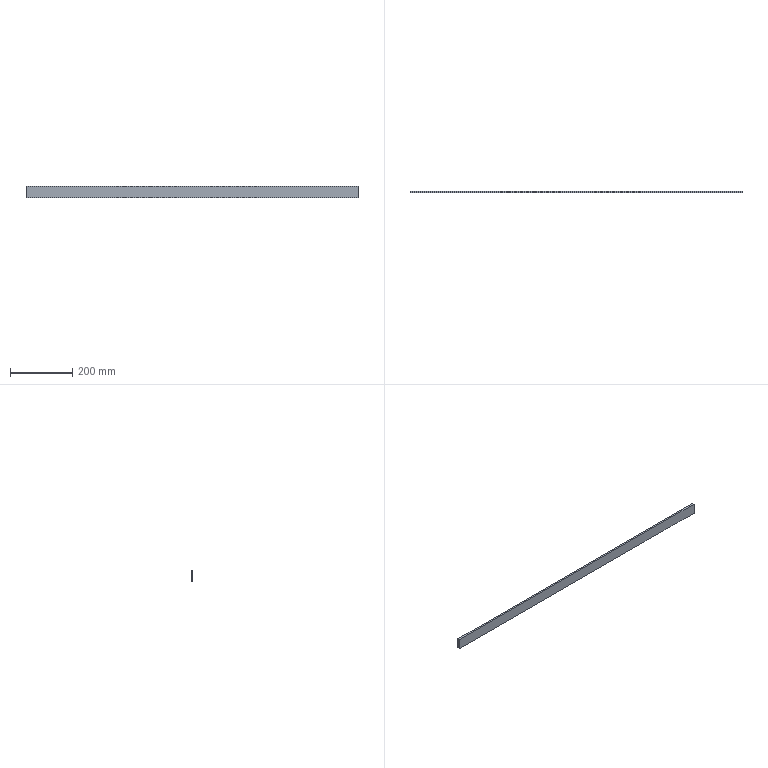Part | STEP file | Pressure plate 1069X36X6_Default<As machined> | 1 solid | 6 faces | box 1069 x 6 x 36 mm | volume 230904 mm3 | plane 6
STEP:
#1=CARTESIAN_POINT('',(0.,0.,0.));
#2=DIRECTION('',(0.,0.,1.));
#3=DIRECTION('',(1.,0.,0.));
#4=AXIS2_PLACEMENT_3D('',#1,#2,#3);
#5=CARTESIAN_POINT('',(534.5,0.,18.));
#6=VERTEX_POINT('',#5);
#7=CARTESIAN_POINT('',(534.5,0.,-18.));
#8=VERTEX_POINT('',#7);
#9=CARTESIAN_POINT('',(534.5,0.,-18.));
#10=DIRECTION('',(0.,0.,-1.));
#11=VECTOR('',#10,1.);
#12=LINE('',#9,#11);
#13=CARTESIAN_POINT('',(534.5,6.,-18.));
#14=DIRECTION('',(-1.,0.,0.));
#15=DIRECTION('',(0.,0.,1.));
#16=AXIS2_PLACEMENT_3D('',#13,#14,#15);
#17=PLANE('',#16);
#18=CARTESIAN_POINT('',(0.,-6.));
#19=DIRECTION('',(-1.,0.));
#20=VECTOR('',#19,1.);
#21=LINE('',#18,#20);
#22=(GEOMETRIC_REPRESENTATION_CONTEXT(2)PARAMETRIC_REPRESENTATION_CONTEXT()REPRESENTATION_CONTEXT('',''));
#23=DEFINITIONAL_REPRESENTATION('',(#21),#22);
#24=PCURVE('',#17,#23);
#25=CARTESIAN_POINT('',(0.,0.,0.));
#26=DIRECTION('',(0.,1.,0.));
#27=DIRECTION('',(0.,0.,1.));
#28=AXIS2_PLACEMENT_3D('',#25,#26,#27);
#29=PLANE('',#28);
#30=CARTESIAN_POINT('',(-18.,534.5));
#31=DIRECTION('',(-1.,0.));
#32=VECTOR('',#31,1.);
#33=LINE('',#30,#32);
#34=(GEOMETRIC_REPRESENTATION_CONTEXT(2)PARAMETRIC_REPRESENTATION_CONTEXT()REPRESENTATION_CONTEXT('',''));
#35=DEFINITIONAL_REPRESENTATION('',(#33),#34);
#36=PCURVE('',#29,#35);
#37=SURFACE_CURVE('',#12,(#24,#36),.PCURVE_S1.);
#38=EDGE_CURVE('',#6,#8,#37,.T.);
#39=ORIENTED_EDGE('',*,*,#38,.T.);
#40=CARTESIAN_POINT('',(534.5,6.,-18.));
#41=VERTEX_POINT('',#40);
#42=CARTESIAN_POINT('',(534.5,6.,-18.));
#43=DIRECTION('',(0.,-1.,0.));
#44=VECTOR('',#43,1.);
#45=LINE('',#42,#44);
#46=CARTESIAN_POINT('',(0.,0.));
#47=DIRECTION('',(0.,-1.));
#48=VECTOR('',#47,1.);
#49=LINE('',#46,#48);
#50=(GEOMETRIC_REPRESENTATION_CONTEXT(2)PARAMETRIC_REPRESENTATION_CONTEXT()REPRESENTATION_CONTEXT('',''));
#51=DEFINITIONAL_REPRESENTATION('',(#49),#50);
#52=PCURVE('',#17,#51);
#53=CARTESIAN_POINT('',(-534.5,6.,-18.));
#54=DIRECTION('',(0.,0.,1.));
#55=DIRECTION('',(1.,0.,0.));
#56=AXIS2_PLACEMENT_3D('',#53,#54,#55);
#57=PLANE('',#56);
#58=CARTESIAN_POINT('',(1069.,0.));
#59=DIRECTION('',(0.,-1.));
#60=VECTOR('',#59,1.);
#61=LINE('',#58,#60);
#62=(GEOMETRIC_REPRESENTATION_CONTEXT(2)PARAMETRIC_REPRESENTATION_CONTEXT()REPRESENTATION_CONTEXT('',''));
#63=DEFINITIONAL_REPRESENTATION('',(#61),#62);
#64=PCURVE('',#57,#63);
#65=SURFACE_CURVE('',#45,(#52,#64),.PCURVE_S1.);
#66=EDGE_CURVE('',#41,#8,#65,.T.);
#67=ORIENTED_EDGE('',*,*,#66,.F.);
#68=CARTESIAN_POINT('',(534.5,6.,18.));
#69=VERTEX_POINT('',#68);
#70=CARTESIAN_POINT('',(534.5,6.,-18.));
#71=DIRECTION('',(0.,0.,-1.));
#72=VECTOR('',#71,1.);
#73=LINE('',#70,#72);
#74=CARTESIAN_POINT('',(0.,0.));
#75=DIRECTION('',(-1.,0.));
#76=VECTOR('',#75,1.);
#77=LINE('',#74,#76);
#78=(GEOMETRIC_REPRESENTATION_CONTEXT(2)PARAMETRIC_REPRESENTATION_CONTEXT()REPRESENTATION_CONTEXT('',''));
#79=DEFINITIONAL_REPRESENTATION('',(#77),#78);
#80=PCURVE('',#17,#79);
#81=CARTESIAN_POINT('',(0.,6.,0.));
#82=DIRECTION('',(0.,1.,0.));
#83=DIRECTION('',(0.,0.,1.));
#84=AXIS2_PLACEMENT_3D('',#81,#82,#83);
#85=PLANE('',#84);
#86=CARTESIAN_POINT('',(-18.,534.5));
#87=DIRECTION('',(-1.,0.));
#88=VECTOR('',#87,1.);
#89=LINE('',#86,#88);
#90=(GEOMETRIC_REPRESENTATION_CONTEXT(2)PARAMETRIC_REPRESENTATION_CONTEXT()REPRESENTATION_CONTEXT('',''));
#91=DEFINITIONAL_REPRESENTATION('',(#89),#90);
#92=PCURVE('',#85,#91);
#93=SURFACE_CURVE('',#73,(#80,#92),.PCURVE_S1.);
#94=EDGE_CURVE('',#69,#41,#93,.T.);
#95=ORIENTED_EDGE('',*,*,#94,.F.);
#96=CARTESIAN_POINT('',(534.5,6.,18.));
#97=DIRECTION('',(0.,-1.,0.));
#98=VECTOR('',#97,1.);
#99=LINE('',#96,#98);
#100=CARTESIAN_POINT('',(36.,0.));
#101=DIRECTION('',(0.,-1.));
#102=VECTOR('',#101,1.);
#103=LINE('',#100,#102);
#104=(GEOMETRIC_REPRESENTATION_CONTEXT(2)PARAMETRIC_REPRESENTATION_CONTEXT()REPRESENTATION_CONTEXT('',''));
#105=DEFINITIONAL_REPRESENTATION('',(#103),#104);
#106=PCURVE('',#17,#105);
#107=CARTESIAN_POINT('',(-534.5,6.,18.));
#108=DIRECTION('',(0.,0.,-1.));
#109=DIRECTION('',(-1.,0.,0.));
#110=AXIS2_PLACEMENT_3D('',#107,#108,#109);
#111=PLANE('',#110);
#112=CARTESIAN_POINT('',(-1069.,0.));
#113=DIRECTION('',(0.,-1.));
#114=VECTOR('',#113,1.);
#115=LINE('',#112,#114);
#116=(GEOMETRIC_REPRESENTATION_CONTEXT(2)PARAMETRIC_REPRESENTATION_CONTEXT()REPRESENTATION_CONTEXT('',''));
#117=DEFINITIONAL_REPRESENTATION('',(#115),#116);
#118=PCURVE('',#111,#117);
#119=SURFACE_CURVE('',#99,(#106,#118),.PCURVE_S1.);
#120=EDGE_CURVE('',#69,#6,#119,.T.);
#121=ORIENTED_EDGE('',*,*,#120,.T.);
#122=EDGE_LOOP('',(#39,#67,#95,#121));
#123=FACE_BOUND('',#122,.T.);
#124=ADVANCED_FACE('',(#123),#17,.F.);
#125=CARTESIAN_POINT('',(-534.5,0.,-18.));
#126=VERTEX_POINT('',#125);
#127=CARTESIAN_POINT('',(-534.5,0.,-18.));
#128=DIRECTION('',(-1.,0.,0.));
#129=VECTOR('',#128,1.);
#130=LINE('',#127,#129);
#131=CARTESIAN_POINT('',(0.,-6.));
#132=DIRECTION('',(-1.,0.));
#133=VECTOR('',#132,1.);
#134=LINE('',#131,#133);
#135=(GEOMETRIC_REPRESENTATION_CONTEXT(2)PARAMETRIC_REPRESENTATION_CONTEXT()REPRESENTATION_CONTEXT('',''));
#136=DEFINITIONAL_REPRESENTATION('',(#134),#135);
#137=PCURVE('',#57,#136);
#138=CARTESIAN_POINT('',(-18.,-534.5));
#139=DIRECTION('',(0.,-1.));
#140=VECTOR('',#139,1.);
#141=LINE('',#138,#140);
#142=(GEOMETRIC_REPRESENTATION_CONTEXT(2)PARAMETRIC_REPRESENTATION_CONTEXT()REPRESENTATION_CONTEXT('',''));
#143=DEFINITIONAL_REPRESENTATION('',(#141),#142);
#144=PCURVE('',#29,#143);
#145=SURFACE_CURVE('',#130,(#137,#144),.PCURVE_S1.);
#146=EDGE_CURVE('',#8,#126,#145,.T.);
#147=ORIENTED_EDGE('',*,*,#146,.T.);
#148=CARTESIAN_POINT('',(-534.5,6.,-18.));
#149=VERTEX_POINT('',#148);
#150=CARTESIAN_POINT('',(-534.5,6.,-18.));
#151=DIRECTION('',(0.,-1.,0.));
#152=VECTOR('',#151,1.);
#153=LINE('',#150,#152);
#154=CARTESIAN_POINT('',(0.,0.));
#155=DIRECTION('',(0.,-1.));
#156=VECTOR('',#155,1.);
#157=LINE('',#154,#156);
#158=(GEOMETRIC_REPRESENTATION_CONTEXT(2)PARAMETRIC_REPRESENTATION_CONTEXT()REPRESENTATION_CONTEXT('',''));
#159=DEFINITIONAL_REPRESENTATION('',(#157),#158);
#160=PCURVE('',#57,#159);
#161=CARTESIAN_POINT('',(-534.5,6.,-18.));
#162=DIRECTION('',(1.,0.,0.));
#163=DIRECTION('',(0.,0.,-1.));
#164=AXIS2_PLACEMENT_3D('',#161,#162,#163);
#165=PLANE('',#164);
#166=CARTESIAN_POINT('',(0.,0.));
#167=DIRECTION('',(0.,-1.));
#168=VECTOR('',#167,1.);
#169=LINE('',#166,#168);
#170=(GEOMETRIC_REPRESENTATION_CONTEXT(2)PARAMETRIC_REPRESENTATION_CONTEXT()REPRESENTATION_CONTEXT('',''));
#171=DEFINITIONAL_REPRESENTATION('',(#169),#170);
#172=PCURVE('',#165,#171);
#173=SURFACE_CURVE('',#153,(#160,#172),.PCURVE_S1.);
#174=EDGE_CURVE('',#149,#126,#173,.T.);
#175=ORIENTED_EDGE('',*,*,#174,.F.);
#176=CARTESIAN_POINT('',(-534.5,6.,-18.));
#177=DIRECTION('',(-1.,0.,0.));
#178=VECTOR('',#177,1.);
#179=LINE('',#176,#178);
#180=CARTESIAN_POINT('',(0.,0.));
#181=DIRECTION('',(-1.,0.));
#182=VECTOR('',#181,1.);
#183=LINE('',#180,#182);
#184=(GEOMETRIC_REPRESENTATION_CONTEXT(2)PARAMETRIC_REPRESENTATION_CONTEXT()REPRESENTATION_CONTEXT('',''));
#185=DEFINITIONAL_REPRESENTATION('',(#183),#184);
#186=PCURVE('',#57,#185);
#187=CARTESIAN_POINT('',(-18.,-534.5));
#188=DIRECTION('',(0.,-1.));
#189=VECTOR('',#188,1.);
#190=LINE('',#187,#189);
#191=(GEOMETRIC_REPRESENTATION_CONTEXT(2)PARAMETRIC_REPRESENTATION_CONTEXT()REPRESENTATION_CONTEXT('',''));
#192=DEFINITIONAL_REPRESENTATION('',(#190),#191);
#193=PCURVE('',#85,#192);
#194=SURFACE_CURVE('',#179,(#186,#193),.PCURVE_S1.);
#195=EDGE_CURVE('',#41,#149,#194,.T.);
#196=ORIENTED_EDGE('',*,*,#195,.F.);
#197=ORIENTED_EDGE('',*,*,#66,.T.);
#198=EDGE_LOOP('',(#147,#175,#196,#197));
#199=FACE_BOUND('',#198,.T.);
#200=ADVANCED_FACE('',(#199),#57,.F.);
#201=CARTESIAN_POINT('',(-534.5,0.,18.));
#202=VERTEX_POINT('',#201);
#203=CARTESIAN_POINT('',(-534.5,0.,-18.));
#204=DIRECTION('',(0.,0.,1.));
#205=VECTOR('',#204,1.);
#206=LINE('',#203,#205);
#207=CARTESIAN_POINT('',(0.,-6.));
#208=DIRECTION('',(-1.,0.));
#209=VECTOR('',#208,1.);
#210=LINE('',#207,#209);
#211=(GEOMETRIC_REPRESENTATION_CONTEXT(2)PARAMETRIC_REPRESENTATION_CONTEXT()REPRESENTATION_CONTEXT('',''));
#212=DEFINITIONAL_REPRESENTATION('',(#210),#211);
#213=PCURVE('',#165,#212);
#214=CARTESIAN_POINT('',(-18.,-534.5));
#215=DIRECTION('',(1.,0.));
#216=VECTOR('',#215,1.);
#217=LINE('',#214,#216);
#218=(GEOMETRIC_REPRESENTATION_CONTEXT(2)PARAMETRIC_REPRESENTATION_CONTEXT()REPRESENTATION_CONTEXT('',''));
#219=DEFINITIONAL_REPRESENTATION('',(#217),#218);
#220=PCURVE('',#29,#219);
#221=SURFACE_CURVE('',#206,(#213,#220),.PCURVE_S1.);
#222=EDGE_CURVE('',#126,#202,#221,.T.);
#223=ORIENTED_EDGE('',*,*,#222,.T.);
#224=CARTESIAN_POINT('',(-534.5,6.,18.));
#225=VERTEX_POINT('',#224);
#226=CARTESIAN_POINT('',(-534.5,6.,18.));
#227=DIRECTION('',(0.,-1.,0.));
#228=VECTOR('',#227,1.);
#229=LINE('',#226,#228);
#230=CARTESIAN_POINT('',(-36.,0.));
#231=DIRECTION('',(0.,-1.));
#232=VECTOR('',#231,1.);
#233=LINE('',#230,#232);
#234=(GEOMETRIC_REPRESENTATION_CONTEXT(2)PARAMETRIC_REPRESENTATION_CONTEXT()REPRESENTATION_CONTEXT('',''));
#235=DEFINITIONAL_REPRESENTATION('',(#233),#234);
#236=PCURVE('',#165,#235);
#237=CARTESIAN_POINT('',(0.,0.));
#238=DIRECTION('',(0.,-1.));
#239=VECTOR('',#238,1.);
#240=LINE('',#237,#239);
#241=(GEOMETRIC_REPRESENTATION_CONTEXT(2)PARAMETRIC_REPRESENTATION_CONTEXT()REPRESENTATION_CONTEXT('',''));
#242=DEFINITIONAL_REPRESENTATION('',(#240),#241);
#243=PCURVE('',#111,#242);
#244=SURFACE_CURVE('',#229,(#236,#243),.PCURVE_S1.);
#245=EDGE_CURVE('',#225,#202,#244,.T.);
#246=ORIENTED_EDGE('',*,*,#245,.F.);
#247=CARTESIAN_POINT('',(-534.5,6.,-18.));
#248=DIRECTION('',(0.,0.,1.));
#249=VECTOR('',#248,1.);
#250=LINE('',#247,#249);
#251=CARTESIAN_POINT('',(0.,0.));
#252=DIRECTION('',(-1.,0.));
#253=VECTOR('',#252,1.);
#254=LINE('',#251,#253);
#255=(GEOMETRIC_REPRESENTATION_CONTEXT(2)PARAMETRIC_REPRESENTATION_CONTEXT()REPRESENTATION_CONTEXT('',''));
#256=DEFINITIONAL_REPRESENTATION('',(#254),#255);
#257=PCURVE('',#165,#256);
#258=CARTESIAN_POINT('',(-18.,-534.5));
#259=DIRECTION('',(1.,0.));
#260=VECTOR('',#259,1.);
#261=LINE('',#258,#260);
#262=(GEOMETRIC_REPRESENTATION_CONTEXT(2)PARAMETRIC_REPRESENTATION_CONTEXT()REPRESENTATION_CONTEXT('',''));
#263=DEFINITIONAL_REPRESENTATION('',(#261),#262);
#264=PCURVE('',#85,#263);
#265=SURFACE_CURVE('',#250,(#257,#264),.PCURVE_S1.);
#266=EDGE_CURVE('',#149,#225,#265,.T.);
#267=ORIENTED_EDGE('',*,*,#266,.F.);
#268=ORIENTED_EDGE('',*,*,#174,.T.);
#269=EDGE_LOOP('',(#223,#246,#267,#268));
#270=FACE_BOUND('',#269,.T.);
#271=ADVANCED_FACE('',(#270),#165,.F.);
#272=CARTESIAN_POINT('',(-534.5,0.,18.));
#273=DIRECTION('',(1.,0.,0.));
#274=VECTOR('',#273,1.);
#275=LINE('',#272,#274);
#276=CARTESIAN_POINT('',(0.,-6.));
#277=DIRECTION('',(-1.,0.));
#278=VECTOR('',#277,1.);
#279=LINE('',#276,#278);
#280=(GEOMETRIC_REPRESENTATION_CONTEXT(2)PARAMETRIC_REPRESENTATION_CONTEXT()REPRESENTATION_CONTEXT('',''));
#281=DEFINITIONAL_REPRESENTATION('',(#279),#280);
#282=PCURVE('',#111,#281);
#283=CARTESIAN_POINT('',(18.,-534.5));
#284=DIRECTION('',(0.,1.));
#285=VECTOR('',#284,1.);
#286=LINE('',#283,#285);
#287=(GEOMETRIC_REPRESENTATION_CONTEXT(2)PARAMETRIC_REPRESENTATION_CONTEXT()REPRESENTATION_CONTEXT('',''));
#288=DEFINITIONAL_REPRESENTATION('',(#286),#287);
#289=PCURVE('',#29,#288);
#290=SURFACE_CURVE('',#275,(#282,#289),.PCURVE_S1.);
#291=EDGE_CURVE('',#202,#6,#290,.T.);
#292=ORIENTED_EDGE('',*,*,#291,.T.);
#293=ORIENTED_EDGE('',*,*,#120,.F.);
#294=CARTESIAN_POINT('',(-534.5,6.,18.));
#295=DIRECTION('',(1.,0.,0.));
#296=VECTOR('',#295,1.);
#297=LINE('',#294,#296);
#298=CARTESIAN_POINT('',(0.,0.));
#299=DIRECTION('',(-1.,0.));
#300=VECTOR('',#299,1.);
#301=LINE('',#298,#300);
#302=(GEOMETRIC_REPRESENTATION_CONTEXT(2)PARAMETRIC_REPRESENTATION_CONTEXT()REPRESENTATION_CONTEXT('',''));
#303=DEFINITIONAL_REPRESENTATION('',(#301),#302);
#304=PCURVE('',#111,#303);
#305=CARTESIAN_POINT('',(18.,-534.5));
#306=DIRECTION('',(0.,1.));
#307=VECTOR('',#306,1.);
#308=LINE('',#305,#307);
#309=(GEOMETRIC_REPRESENTATION_CONTEXT(2)PARAMETRIC_REPRESENTATION_CONTEXT()REPRESENTATION_CONTEXT('',''));
#310=DEFINITIONAL_REPRESENTATION('',(#308),#309);
#311=PCURVE('',#85,#310);
#312=SURFACE_CURVE('',#297,(#304,#311),.PCURVE_S1.);
#313=EDGE_CURVE('',#225,#69,#312,.T.);
#314=ORIENTED_EDGE('',*,*,#313,.F.);
#315=ORIENTED_EDGE('',*,*,#245,.T.);
#316=EDGE_LOOP('',(#292,#293,#314,#315));
#317=FACE_BOUND('',#316,.T.);
#318=ADVANCED_FACE('',(#317),#111,.F.);
#319=ORIENTED_EDGE('',*,*,#94,.T.);
#320=ORIENTED_EDGE('',*,*,#195,.T.);
#321=ORIENTED_EDGE('',*,*,#266,.T.);
#322=ORIENTED_EDGE('',*,*,#313,.T.);
#323=EDGE_LOOP('',(#319,#320,#321,#322));
#324=FACE_BOUND('',#323,.T.);
#325=ADVANCED_FACE('',(#324),#85,.T.);
#326=ORIENTED_EDGE('',*,*,#38,.F.);
#327=ORIENTED_EDGE('',*,*,#291,.F.);
#328=ORIENTED_EDGE('',*,*,#222,.F.);
#329=ORIENTED_EDGE('',*,*,#146,.F.);
#330=EDGE_LOOP('',(#326,#327,#328,#329));
#331=FACE_BOUND('',#330,.T.);
#332=ADVANCED_FACE('',(#331),#29,.F.);
#333=CLOSED_SHELL('',(#124,#200,#271,#318,#325,#332));
#334=MANIFOLD_SOLID_BREP('',#333);
#335=(LENGTH_UNIT()NAMED_UNIT(*)SI_UNIT(.MILLI.,.METRE.));
#336=UNCERTAINTY_MEASURE_WITH_UNIT(LENGTH_MEASURE(0.0000001),#335,'','');
#337=(NAMED_UNIT(*)PLANE_ANGLE_UNIT()SI_UNIT($,.RADIAN.));
#338=(NAMED_UNIT(*)SI_UNIT($,.STERADIAN.)SOLID_ANGLE_UNIT());
#339=(GEOMETRIC_REPRESENTATION_CONTEXT(3)GLOBAL_UNCERTAINTY_ASSIGNED_CONTEXT((#336))GLOBAL_UNIT_ASSIGNED_CONTEXT((#335,#337,#338))REPRESENTATION_CONTEXT('',''));
#340=ADVANCED_BREP_SHAPE_REPRESENTATION('',(#4,#334),#339);